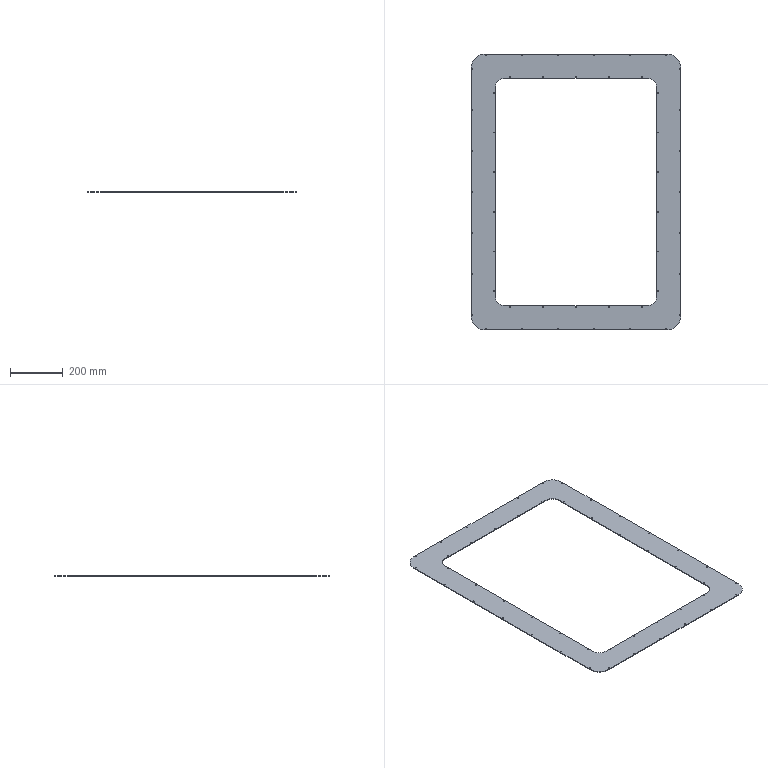Part | STEP file | HESS-408-70-15W-N-13-inner liner outer closing plate | 1 solid | 114 faces | box 792 x 1042 x 2.5 mm | volume 754601 mm3 | cylinder 104 | plane 10 | commonest cylinder face diameters 3.2 x96 60 x4 100 x4